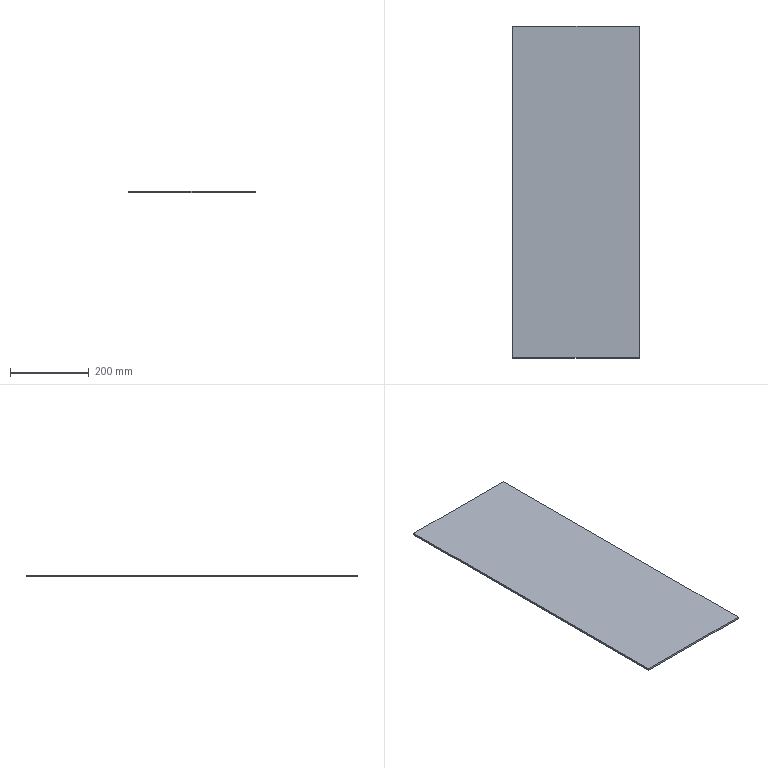Part | SolidWorks | features Extrusion 1, HoleWzd 1 | 1 solid | 6 faces | box 321 x 842 x 5 mm | volume 1351410 mm3 | plane 6
STEP:
#1=CARTESIAN_POINT('',(160.5,-421.,0.));
#2=VERTEX_POINT('',#1);
#3=CARTESIAN_POINT('',(160.5,421.,0.));
#4=VERTEX_POINT('',#3);
#5=CARTESIAN_POINT('',(160.5,421.,0.));
#6=DIRECTION('',(0.,1.,0.));
#7=VECTOR('',#6,1000.);
#8=LINE('',#5,#7);
#9=EDGE_CURVE('',#2,#4,#8,.T.);
#10=ORIENTED_EDGE('',*,*,#9,.T.);
#11=CARTESIAN_POINT('',(160.5,421.,5.));
#12=VERTEX_POINT('',#11);
#13=CARTESIAN_POINT('',(160.5,421.,5.));
#14=DIRECTION('',(0.,0.,-1.));
#15=VECTOR('',#14,1000.);
#16=LINE('',#13,#15);
#17=EDGE_CURVE('',#12,#4,#16,.T.);
#18=ORIENTED_EDGE('',*,*,#17,.F.);
#19=CARTESIAN_POINT('',(160.5,-421.,5.));
#20=VERTEX_POINT('',#19);
#21=CARTESIAN_POINT('',(160.5,421.,5.));
#22=DIRECTION('',(0.,1.,0.));
#23=VECTOR('',#22,1000.);
#24=LINE('',#21,#23);
#25=EDGE_CURVE('',#20,#12,#24,.T.);
#26=ORIENTED_EDGE('',*,*,#25,.F.);
#27=CARTESIAN_POINT('',(160.5,-421.,5.));
#28=DIRECTION('',(0.,0.,-1.));
#29=VECTOR('',#28,1000.);
#30=LINE('',#27,#29);
#31=EDGE_CURVE('',#20,#2,#30,.T.);
#32=ORIENTED_EDGE('',*,*,#31,.T.);
#33=EDGE_LOOP('',(#10,#18,#26,#32));
#34=FACE_OUTER_BOUND('',#33,.T.);
#35=CARTESIAN_POINT('',(160.5,421.,5.));
#36=DIRECTION('',(-1.,0.,0.));
#37=DIRECTION('',(0.,-1.,0.));
#38=AXIS2_PLACEMENT_3D('',#35,#36,#37);
#39=PLANE('',#38);
#40=ADVANCED_FACE('',(#34),#39,.F.);
#41=CARTESIAN_POINT('',(-160.5,421.,0.));
#42=VERTEX_POINT('',#41);
#43=CARTESIAN_POINT('',(-160.5,421.,0.));
#44=DIRECTION('',(-1.,0.,0.));
#45=VECTOR('',#44,1000.);
#46=LINE('',#43,#45);
#47=EDGE_CURVE('',#4,#42,#46,.T.);
#48=ORIENTED_EDGE('',*,*,#47,.T.);
#49=CARTESIAN_POINT('',(-160.5,421.,5.));
#50=VERTEX_POINT('',#49);
#51=CARTESIAN_POINT('',(-160.5,421.,5.));
#52=DIRECTION('',(0.,0.,-1.));
#53=VECTOR('',#52,1000.);
#54=LINE('',#51,#53);
#55=EDGE_CURVE('',#50,#42,#54,.T.);
#56=ORIENTED_EDGE('',*,*,#55,.F.);
#57=CARTESIAN_POINT('',(-160.5,421.,5.));
#58=DIRECTION('',(-1.,0.,0.));
#59=VECTOR('',#58,1000.);
#60=LINE('',#57,#59);
#61=EDGE_CURVE('',#12,#50,#60,.T.);
#62=ORIENTED_EDGE('',*,*,#61,.F.);
#63=ORIENTED_EDGE('',*,*,#17,.T.);
#64=EDGE_LOOP('',(#48,#56,#62,#63));
#65=FACE_OUTER_BOUND('',#64,.T.);
#66=CARTESIAN_POINT('',(-160.5,421.,5.));
#67=DIRECTION('',(0.,-1.,0.));
#68=DIRECTION('',(0.,0.,-1.));
#69=AXIS2_PLACEMENT_3D('',#66,#67,#68);
#70=PLANE('',#69);
#71=ADVANCED_FACE('',(#65),#70,.F.);
#72=CARTESIAN_POINT('',(-160.5,-421.,0.));
#73=VERTEX_POINT('',#72);
#74=CARTESIAN_POINT('',(-160.5,421.,0.));
#75=DIRECTION('',(0.,-1.,0.));
#76=VECTOR('',#75,1000.);
#77=LINE('',#74,#76);
#78=EDGE_CURVE('',#42,#73,#77,.T.);
#79=ORIENTED_EDGE('',*,*,#78,.T.);
#80=CARTESIAN_POINT('',(-160.5,-421.,5.));
#81=VERTEX_POINT('',#80);
#82=CARTESIAN_POINT('',(-160.5,-421.,5.));
#83=DIRECTION('',(0.,0.,-1.));
#84=VECTOR('',#83,1000.);
#85=LINE('',#82,#84);
#86=EDGE_CURVE('',#81,#73,#85,.T.);
#87=ORIENTED_EDGE('',*,*,#86,.F.);
#88=CARTESIAN_POINT('',(-160.5,421.,5.));
#89=DIRECTION('',(0.,-1.,0.));
#90=VECTOR('',#89,1000.);
#91=LINE('',#88,#90);
#92=EDGE_CURVE('',#50,#81,#91,.T.);
#93=ORIENTED_EDGE('',*,*,#92,.F.);
#94=ORIENTED_EDGE('',*,*,#55,.T.);
#95=EDGE_LOOP('',(#79,#87,#93,#94));
#96=FACE_OUTER_BOUND('',#95,.T.);
#97=CARTESIAN_POINT('',(-160.5,421.,5.));
#98=DIRECTION('',(1.,0.,0.));
#99=DIRECTION('',(0.,1.,0.));
#100=AXIS2_PLACEMENT_3D('',#97,#98,#99);
#101=PLANE('',#100);
#102=ADVANCED_FACE('',(#96),#101,.F.);
#103=CARTESIAN_POINT('',(-160.5,-421.,0.));
#104=DIRECTION('',(1.,0.,0.));
#105=VECTOR('',#104,1000.);
#106=LINE('',#103,#105);
#107=EDGE_CURVE('',#73,#2,#106,.T.);
#108=ORIENTED_EDGE('',*,*,#107,.T.);
#109=ORIENTED_EDGE('',*,*,#31,.F.);
#110=CARTESIAN_POINT('',(-160.5,-421.,5.));
#111=DIRECTION('',(1.,0.,0.));
#112=VECTOR('',#111,1000.);
#113=LINE('',#110,#112);
#114=EDGE_CURVE('',#81,#20,#113,.T.);
#115=ORIENTED_EDGE('',*,*,#114,.F.);
#116=ORIENTED_EDGE('',*,*,#86,.T.);
#117=EDGE_LOOP('',(#108,#109,#115,#116));
#118=FACE_OUTER_BOUND('',#117,.T.);
#119=CARTESIAN_POINT('',(-160.5,-421.,5.));
#120=DIRECTION('',(0.,1.,0.));
#121=DIRECTION('',(0.,0.,1.));
#122=AXIS2_PLACEMENT_3D('',#119,#120,#121);
#123=PLANE('',#122);
#124=ADVANCED_FACE('',(#118),#123,.F.);
#125=ORIENTED_EDGE('',*,*,#25,.T.);
#126=ORIENTED_EDGE('',*,*,#61,.T.);
#127=ORIENTED_EDGE('',*,*,#92,.T.);
#128=ORIENTED_EDGE('',*,*,#114,.T.);
#129=EDGE_LOOP('',(#125,#126,#127,#128));
#130=FACE_OUTER_BOUND('',#129,.T.);
#131=CARTESIAN_POINT('',(0.,0.,5.));
#132=DIRECTION('',(0.,0.,1.));
#133=DIRECTION('',(1.,0.,0.));
#134=AXIS2_PLACEMENT_3D('',#131,#132,#133);
#135=PLANE('',#134);
#136=ADVANCED_FACE('',(#130),#135,.T.);
#137=ORIENTED_EDGE('',*,*,#9,.F.);
#138=ORIENTED_EDGE('',*,*,#107,.F.);
#139=ORIENTED_EDGE('',*,*,#78,.F.);
#140=ORIENTED_EDGE('',*,*,#47,.F.);
#141=EDGE_LOOP('',(#137,#138,#139,#140));
#142=FACE_OUTER_BOUND('',#141,.T.);
#143=CARTESIAN_POINT('',(0.,0.,0.));
#144=DIRECTION('',(0.,0.,1.));
#145=DIRECTION('',(1.,0.,0.));
#146=AXIS2_PLACEMENT_3D('',#143,#144,#145);
#147=PLANE('',#146);
#148=ADVANCED_FACE('',(#142),#147,.F.);
#149=CLOSED_SHELL('',(#40,#71,#102,#124,#136,#148));
#150=MANIFOLD_SOLID_BREP('',#149);
#151=CARTESIAN_POINT('',(0.,0.,0.));
#152=DIRECTION('',(0.,0.,1.));
#153=DIRECTION('',(1.,0.,0.));
#154=AXIS2_PLACEMENT_3D('',#151,#152,#153);
#155=(LENGTH_UNIT()NAMED_UNIT(*)SI_UNIT(.MILLI.,.METRE.));
#156=UNCERTAINTY_MEASURE_WITH_UNIT(LENGTH_MEASURE(0.00001),#155,'','');
#157=(NAMED_UNIT(*)PLANE_ANGLE_UNIT()SI_UNIT($,.RADIAN.));
#158=(NAMED_UNIT(*)SI_UNIT($,.STERADIAN.)SOLID_ANGLE_UNIT());
#159=(GEOMETRIC_REPRESENTATION_CONTEXT(3)GLOBAL_UNCERTAINTY_ASSIGNED_CONTEXT((#156))GLOBAL_UNIT_ASSIGNED_CONTEXT((#155,#157,#158))REPRESENTATION_CONTEXT('',''));
#160=ADVANCED_BREP_SHAPE_REPRESENTATION('',(#150,#154),#159);